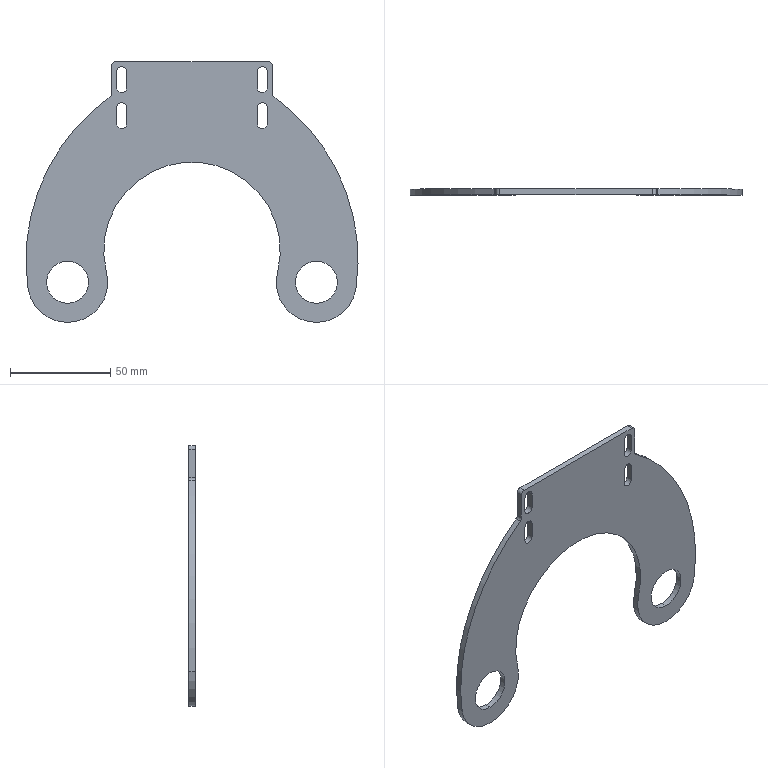Part | 1 solid | 40 faces | box 165.52 x 3 x 130 mm | volume 31712 mm3 | cylinder 27 | plane 13 | commonest cylinder face diameters 5 x12 4 x4 21 x4 40 x4 200 x2 88 x1
STEP:
#1=CARTESIAN_POINT('',(5.,0.,-2.5));
#2=VERTEX_POINT('',#1);
#3=CARTESIAN_POINT('',(7.5,0.,-5.));
#4=VERTEX_POINT('',#3);
#5=CARTESIAN_POINT('',(5.,0.,-5.));
#6=DIRECTION('',(0.,1.,0.));
#7=DIRECTION('',(0.,0.,1.));
#8=AXIS2_PLACEMENT_3D('',#5,#6,#7);
#9=CIRCLE('',#8,2.5);
#10=EDGE_CURVE('',#2,#4,#9,.T.);
#11=ORIENTED_EDGE('',*,*,#10,.F.);
#12=CARTESIAN_POINT('',(5.,3.,-2.5));
#13=VERTEX_POINT('',#12);
#14=CARTESIAN_POINT('',(5.,0.,-2.5));
#15=DIRECTION('',(0.,1.,0.));
#16=VECTOR('',#15,1000.);
#17=LINE('',#14,#16);
#18=EDGE_CURVE('',#2,#13,#17,.T.);
#19=ORIENTED_EDGE('',*,*,#18,.T.);
#20=CARTESIAN_POINT('',(7.5,3.,-5.));
#21=VERTEX_POINT('',#20);
#22=CARTESIAN_POINT('',(5.,3.,-5.));
#23=DIRECTION('',(0.,1.,0.));
#24=DIRECTION('',(0.,0.,1.));
#25=AXIS2_PLACEMENT_3D('',#22,#23,#24);
#26=CIRCLE('',#25,2.5);
#27=EDGE_CURVE('',#13,#21,#26,.T.);
#28=ORIENTED_EDGE('',*,*,#27,.T.);
#29=CARTESIAN_POINT('',(7.5,0.,-5.));
#30=DIRECTION('',(0.,1.,0.));
#31=VECTOR('',#30,1000.);
#32=LINE('',#29,#31);
#33=EDGE_CURVE('',#4,#21,#32,.T.);
#34=ORIENTED_EDGE('',*,*,#33,.F.);
#35=EDGE_LOOP('',(#11,#19,#28,#34));
#36=FACE_OUTER_BOUND('',#35,.T.);
#37=CARTESIAN_POINT('',(5.,0.,-5.));
#38=DIRECTION('',(0.,1.,0.));
#39=DIRECTION('',(0.,0.,1.));
#40=AXIS2_PLACEMENT_3D('',#37,#38,#39);
#41=CYLINDRICAL_SURFACE('',#40,2.5);
#42=ADVANCED_FACE('',(#36),#41,.F.);
#43=CARTESIAN_POINT('',(75.,0.,-20.5));
#44=VERTEX_POINT('',#43);
#45=CARTESIAN_POINT('',(77.5,0.,-23.));
#46=VERTEX_POINT('',#45);
#47=CARTESIAN_POINT('',(75.,0.,-23.));
#48=DIRECTION('',(0.,1.,0.));
#49=DIRECTION('',(0.,0.,-1.));
#50=AXIS2_PLACEMENT_3D('',#47,#48,#49);
#51=CIRCLE('',#50,2.5);
#52=EDGE_CURVE('',#44,#46,#51,.T.);
#53=ORIENTED_EDGE('',*,*,#52,.F.);
#54=CARTESIAN_POINT('',(75.,3.,-20.5));
#55=VERTEX_POINT('',#54);
#56=CARTESIAN_POINT('',(75.,0.,-20.5));
#57=DIRECTION('',(0.,1.,0.));
#58=VECTOR('',#57,1000.);
#59=LINE('',#56,#58);
#60=EDGE_CURVE('',#44,#55,#59,.T.);
#61=ORIENTED_EDGE('',*,*,#60,.T.);
#62=CARTESIAN_POINT('',(77.5,3.,-23.));
#63=VERTEX_POINT('',#62);
#64=CARTESIAN_POINT('',(75.,3.,-23.));
#65=DIRECTION('',(0.,1.,0.));
#66=DIRECTION('',(0.,0.,-1.));
#67=AXIS2_PLACEMENT_3D('',#64,#65,#66);
#68=CIRCLE('',#67,2.5);
#69=EDGE_CURVE('',#55,#63,#68,.T.);
#70=ORIENTED_EDGE('',*,*,#69,.T.);
#71=CARTESIAN_POINT('',(77.5,0.,-23.));
#72=DIRECTION('',(0.,1.,0.));
#73=VECTOR('',#72,1000.);
#74=LINE('',#71,#73);
#75=EDGE_CURVE('',#46,#63,#74,.T.);
#76=ORIENTED_EDGE('',*,*,#75,.F.);
#77=EDGE_LOOP('',(#53,#61,#70,#76));
#78=FACE_OUTER_BOUND('',#77,.T.);
#79=CARTESIAN_POINT('',(75.,0.,-23.));
#80=DIRECTION('',(0.,1.,0.));
#81=DIRECTION('',(0.,0.,1.));
#82=AXIS2_PLACEMENT_3D('',#79,#80,#81);
#83=CYLINDRICAL_SURFACE('',#82,2.5);
#84=ADVANCED_FACE('',(#78),#83,.F.);
#85=CARTESIAN_POINT('',(75.,0.,-2.5));
#86=VERTEX_POINT('',#85);
#87=CARTESIAN_POINT('',(77.5,0.,-5.));
#88=VERTEX_POINT('',#87);
#89=CARTESIAN_POINT('',(75.,0.,-5.));
#90=DIRECTION('',(0.,1.,0.));
#91=DIRECTION('',(0.,0.,-1.));
#92=AXIS2_PLACEMENT_3D('',#89,#90,#91);
#93=CIRCLE('',#92,2.5);
#94=EDGE_CURVE('',#86,#88,#93,.T.);
#95=ORIENTED_EDGE('',*,*,#94,.F.);
#96=CARTESIAN_POINT('',(75.,3.,-2.5));
#97=VERTEX_POINT('',#96);
#98=CARTESIAN_POINT('',(75.,0.,-2.5));
#99=DIRECTION('',(0.,1.,0.));
#100=VECTOR('',#99,1000.);
#101=LINE('',#98,#100);
#102=EDGE_CURVE('',#86,#97,#101,.T.);
#103=ORIENTED_EDGE('',*,*,#102,.T.);
#104=CARTESIAN_POINT('',(77.5,3.,-5.));
#105=VERTEX_POINT('',#104);
#106=CARTESIAN_POINT('',(75.,3.,-5.));
#107=DIRECTION('',(0.,1.,0.));
#108=DIRECTION('',(0.,0.,-1.));
#109=AXIS2_PLACEMENT_3D('',#106,#107,#108);
#110=CIRCLE('',#109,2.5);
#111=EDGE_CURVE('',#97,#105,#110,.T.);
#112=ORIENTED_EDGE('',*,*,#111,.T.);
#113=CARTESIAN_POINT('',(77.5,0.,-5.));
#114=DIRECTION('',(0.,1.,0.));
#115=VECTOR('',#114,1000.);
#116=LINE('',#113,#115);
#117=EDGE_CURVE('',#88,#105,#116,.T.);
#118=ORIENTED_EDGE('',*,*,#117,.F.);
#119=EDGE_LOOP('',(#95,#103,#112,#118));
#120=FACE_OUTER_BOUND('',#119,.T.);
#121=CARTESIAN_POINT('',(75.,0.,-5.));
#122=DIRECTION('',(0.,1.,0.));
#123=DIRECTION('',(0.,0.,1.));
#124=AXIS2_PLACEMENT_3D('',#121,#122,#123);
#125=CYLINDRICAL_SURFACE('',#124,2.5);
#126=ADVANCED_FACE('',(#120),#125,.F.);
#127=CARTESIAN_POINT('',(5.,0.,-20.5));
#128=VERTEX_POINT('',#127);
#129=CARTESIAN_POINT('',(7.5,0.,-23.));
#130=VERTEX_POINT('',#129);
#131=CARTESIAN_POINT('',(5.,0.,-23.));
#132=DIRECTION('',(0.,1.,0.));
#133=DIRECTION('',(0.,0.,1.));
#134=AXIS2_PLACEMENT_3D('',#131,#132,#133);
#135=CIRCLE('',#134,2.5);
#136=EDGE_CURVE('',#128,#130,#135,.T.);
#137=ORIENTED_EDGE('',*,*,#136,.F.);
#138=CARTESIAN_POINT('',(5.,3.,-20.5));
#139=VERTEX_POINT('',#138);
#140=CARTESIAN_POINT('',(5.,0.,-20.5));
#141=DIRECTION('',(0.,1.,0.));
#142=VECTOR('',#141,1000.);
#143=LINE('',#140,#142);
#144=EDGE_CURVE('',#128,#139,#143,.T.);
#145=ORIENTED_EDGE('',*,*,#144,.T.);
#146=CARTESIAN_POINT('',(7.5,3.,-23.));
#147=VERTEX_POINT('',#146);
#148=CARTESIAN_POINT('',(5.,3.,-23.));
#149=DIRECTION('',(0.,1.,0.));
#150=DIRECTION('',(0.,0.,1.));
#151=AXIS2_PLACEMENT_3D('',#148,#149,#150);
#152=CIRCLE('',#151,2.5);
#153=EDGE_CURVE('',#139,#147,#152,.T.);
#154=ORIENTED_EDGE('',*,*,#153,.T.);
#155=CARTESIAN_POINT('',(7.5,0.,-23.));
#156=DIRECTION('',(0.,1.,0.));
#157=VECTOR('',#156,1000.);
#158=LINE('',#155,#157);
#159=EDGE_CURVE('',#130,#147,#158,.T.);
#160=ORIENTED_EDGE('',*,*,#159,.F.);
#161=EDGE_LOOP('',(#137,#145,#154,#160));
#162=FACE_OUTER_BOUND('',#161,.T.);
#163=CARTESIAN_POINT('',(5.,0.,-23.));
#164=DIRECTION('',(0.,1.,0.));
#165=DIRECTION('',(0.,0.,1.));
#166=AXIS2_PLACEMENT_3D('',#163,#164,#165);
#167=CYLINDRICAL_SURFACE('',#166,2.5);
#168=ADVANCED_FACE('',(#162),#167,.F.);
#169=CARTESIAN_POINT('',(-22.,0.,-120.5));
#170=VERTEX_POINT('',#169);
#171=CARTESIAN_POINT('',(-22.,0.,-99.5));
#172=VERTEX_POINT('',#171);
#173=CARTESIAN_POINT('',(-22.,0.,-110.));
#174=DIRECTION('',(0.,1.,0.));
#175=DIRECTION('',(0.,0.,1.));
#176=AXIS2_PLACEMENT_3D('',#173,#174,#175);
#177=CIRCLE('',#176,10.5);
#178=EDGE_CURVE('',#170,#172,#177,.T.);
#179=ORIENTED_EDGE('',*,*,#178,.F.);
#180=CARTESIAN_POINT('',(-22.,3.,-120.5));
#181=VERTEX_POINT('',#180);
#182=CARTESIAN_POINT('',(-22.,3.,-120.5));
#183=DIRECTION('',(0.,1.,0.));
#184=VECTOR('',#183,1000.);
#185=LINE('',#182,#184);
#186=EDGE_CURVE('',#170,#181,#185,.T.);
#187=ORIENTED_EDGE('',*,*,#186,.T.);
#188=CARTESIAN_POINT('',(-22.,3.,-99.5));
#189=VERTEX_POINT('',#188);
#190=CARTESIAN_POINT('',(-22.,3.,-110.));
#191=DIRECTION('',(0.,1.,0.));
#192=DIRECTION('',(0.,0.,1.));
#193=AXIS2_PLACEMENT_3D('',#190,#191,#192);
#194=CIRCLE('',#193,10.5);
#195=EDGE_CURVE('',#181,#189,#194,.T.);
#196=ORIENTED_EDGE('',*,*,#195,.T.);
#197=CARTESIAN_POINT('',(-22.,3.,-99.5));
#198=DIRECTION('',(0.,1.,0.));
#199=VECTOR('',#198,1000.);
#200=LINE('',#197,#199);
#201=EDGE_CURVE('',#172,#189,#200,.T.);
#202=ORIENTED_EDGE('',*,*,#201,.F.);
#203=EDGE_LOOP('',(#179,#187,#196,#202));
#204=FACE_OUTER_BOUND('',#203,.T.);
#205=CARTESIAN_POINT('',(-22.,3.,-110.));
#206=DIRECTION('',(0.,1.,0.));
#207=DIRECTION('',(0.,0.,1.));
#208=AXIS2_PLACEMENT_3D('',#205,#206,#207);
#209=CYLINDRICAL_SURFACE('',#208,10.5);
#210=ADVANCED_FACE('',(#204),#209,.F.);
#211=CARTESIAN_POINT('',(102.,0.,-120.5));
#212=VERTEX_POINT('',#211);
#213=CARTESIAN_POINT('',(102.,0.,-99.5));
#214=VERTEX_POINT('',#213);
#215=CARTESIAN_POINT('',(102.,0.,-110.));
#216=DIRECTION('',(0.,1.,0.));
#217=DIRECTION('',(0.,0.,1.));
#218=AXIS2_PLACEMENT_3D('',#215,#216,#217);
#219=CIRCLE('',#218,10.5);
#220=EDGE_CURVE('',#212,#214,#219,.T.);
#221=ORIENTED_EDGE('',*,*,#220,.F.);
#222=CARTESIAN_POINT('',(102.,3.,-120.5));
#223=VERTEX_POINT('',#222);
#224=CARTESIAN_POINT('',(102.,3.,-120.5));
#225=DIRECTION('',(0.,1.,0.));
#226=VECTOR('',#225,1000.);
#227=LINE('',#224,#226);
#228=EDGE_CURVE('',#212,#223,#227,.T.);
#229=ORIENTED_EDGE('',*,*,#228,.T.);
#230=CARTESIAN_POINT('',(102.,3.,-99.5));
#231=VERTEX_POINT('',#230);
#232=CARTESIAN_POINT('',(102.,3.,-110.));
#233=DIRECTION('',(0.,1.,0.));
#234=DIRECTION('',(0.,0.,1.));
#235=AXIS2_PLACEMENT_3D('',#232,#233,#234);
#236=CIRCLE('',#235,10.5);
#237=EDGE_CURVE('',#223,#231,#236,.T.);
#238=ORIENTED_EDGE('',*,*,#237,.T.);
#239=CARTESIAN_POINT('',(102.,3.,-99.5));
#240=DIRECTION('',(0.,1.,0.));
#241=VECTOR('',#240,1000.);
#242=LINE('',#239,#241);
#243=EDGE_CURVE('',#214,#231,#242,.T.);
#244=ORIENTED_EDGE('',*,*,#243,.F.);
#245=EDGE_LOOP('',(#221,#229,#238,#244));
#246=FACE_OUTER_BOUND('',#245,.T.);
#247=CARTESIAN_POINT('',(102.,3.,-110.));
#248=DIRECTION('',(0.,1.,0.));
#249=DIRECTION('',(0.,0.,1.));
#250=AXIS2_PLACEMENT_3D('',#247,#248,#249);
#251=CYLINDRICAL_SURFACE('',#250,10.5);
#252=ADVANCED_FACE('',(#246),#251,.F.);
#253=CARTESIAN_POINT('',(-22.,3.,-130.));
#254=VERTEX_POINT('',#253);
#255=CARTESIAN_POINT('',(-41.81,3.,-112.751));
#256=VERTEX_POINT('',#255);
#257=CARTESIAN_POINT('',(-22.,3.,-110.));
#258=DIRECTION('',(0.,1.,0.));
#259=DIRECTION('',(0.,0.,1.));
#260=AXIS2_PLACEMENT_3D('',#257,#258,#259);
#261=CIRCLE('',#260,20.);
#262=EDGE_CURVE('',#254,#256,#261,.T.);
#263=ORIENTED_EDGE('',*,*,#262,.F.);
#264=CARTESIAN_POINT('',(-22.,0.,-130.));
#265=VERTEX_POINT('',#264);
#266=CARTESIAN_POINT('',(-22.,3.,-130.));
#267=DIRECTION('',(0.,-1.,0.));
#268=VECTOR('',#267,1000.);
#269=LINE('',#266,#268);
#270=EDGE_CURVE('',#254,#265,#269,.T.);
#271=ORIENTED_EDGE('',*,*,#270,.T.);
#272=CARTESIAN_POINT('',(-41.81,0.,-112.751));
#273=VERTEX_POINT('',#272);
#274=CARTESIAN_POINT('',(-22.,0.,-110.));
#275=DIRECTION('',(0.,1.,0.));
#276=DIRECTION('',(0.,0.,1.));
#277=AXIS2_PLACEMENT_3D('',#274,#275,#276);
#278=CIRCLE('',#277,20.);
#279=EDGE_CURVE('',#265,#273,#278,.T.);
#280=ORIENTED_EDGE('',*,*,#279,.T.);
#281=CARTESIAN_POINT('',(-41.81,3.,-112.751));
#282=DIRECTION('',(0.,-1.,0.));
#283=VECTOR('',#282,1000.);
#284=LINE('',#281,#283);
#285=EDGE_CURVE('',#256,#273,#284,.T.);
#286=ORIENTED_EDGE('',*,*,#285,.F.);
#287=EDGE_LOOP('',(#263,#271,#280,#286));
#288=FACE_OUTER_BOUND('',#287,.T.);
#289=CARTESIAN_POINT('',(-22.,3.,-110.));
#290=DIRECTION('',(0.,-1.,0.));
#291=DIRECTION('',(0.,0.,-1.));
#292=AXIS2_PLACEMENT_3D('',#289,#290,#291);
#293=CYLINDRICAL_SURFACE('',#292,20.);
#294=ADVANCED_FACE('',(#288),#293,.T.);
#295=CARTESIAN_POINT('',(102.,3.,-130.));
#296=VERTEX_POINT('',#295);
#297=CARTESIAN_POINT('',(82.625,3.,-105.039));
#298=VERTEX_POINT('',#297);
#299=CARTESIAN_POINT('',(102.,3.,-110.));
#300=DIRECTION('',(0.,1.,0.));
#301=DIRECTION('',(0.,0.,-1.));
#302=AXIS2_PLACEMENT_3D('',#299,#300,#301);
#303=CIRCLE('',#302,20.);
#304=EDGE_CURVE('',#296,#298,#303,.T.);
#305=ORIENTED_EDGE('',*,*,#304,.F.);
#306=CARTESIAN_POINT('',(102.,0.,-130.));
#307=VERTEX_POINT('',#306);
#308=CARTESIAN_POINT('',(102.,3.,-130.));
#309=DIRECTION('',(0.,-1.,0.));
#310=VECTOR('',#309,1000.);
#311=LINE('',#308,#310);
#312=EDGE_CURVE('',#296,#307,#311,.T.);
#313=ORIENTED_EDGE('',*,*,#312,.T.);
#314=CARTESIAN_POINT('',(82.625,0.,-105.039));
#315=VERTEX_POINT('',#314);
#316=CARTESIAN_POINT('',(102.,0.,-110.));
#317=DIRECTION('',(0.,1.,0.));
#318=DIRECTION('',(0.,0.,-1.));
#319=AXIS2_PLACEMENT_3D('',#316,#317,#318);
#320=CIRCLE('',#319,20.);
#321=EDGE_CURVE('',#307,#315,#320,.T.);
#322=ORIENTED_EDGE('',*,*,#321,.T.);
#323=CARTESIAN_POINT('',(82.625,3.,-105.039));
#324=DIRECTION('',(0.,-1.,0.));
#325=VECTOR('',#324,1000.);
#326=LINE('',#323,#325);
#327=EDGE_CURVE('',#298,#315,#326,.T.);
#328=ORIENTED_EDGE('',*,*,#327,.F.);
#329=EDGE_LOOP('',(#305,#313,#322,#328));
#330=FACE_OUTER_BOUND('',#329,.T.);
#331=CARTESIAN_POINT('',(102.,3.,-110.));
#332=DIRECTION('',(0.,-1.,0.));
#333=DIRECTION('',(0.,0.,-1.));
#334=AXIS2_PLACEMENT_3D('',#331,#332,#333);
#335=CYLINDRICAL_SURFACE('',#334,20.);
#336=ADVANCED_FACE('',(#330),#335,.T.);
#337=CARTESIAN_POINT('',(0.,0.,-15.964));
#338=VERTEX_POINT('',#337);
#339=CARTESIAN_POINT('',(0.,0.,-2.));
#340=VERTEX_POINT('',#339);
#341=CARTESIAN_POINT('',(0.,0.,0.));
#342=DIRECTION('',(0.,0.,1.));
#343=VECTOR('',#342,1000.);
#344=LINE('',#341,#343);
#345=EDGE_CURVE('',#338,#340,#344,.T.);
#346=ORIENTED_EDGE('',*,*,#345,.T.);
#347=CARTESIAN_POINT('',(0.,3.,-2.));
#348=VERTEX_POINT('',#347);
#349=CARTESIAN_POINT('',(0.,3.,-2.));
#350=DIRECTION('',(0.,1.,0.));
#351=VECTOR('',#350,1000.);
#352=LINE('',#349,#351);
#353=EDGE_CURVE('',#340,#348,#352,.T.);
#354=ORIENTED_EDGE('',*,*,#353,.T.);
#355=CARTESIAN_POINT('',(0.,3.,-15.964));
#356=VERTEX_POINT('',#355);
#357=CARTESIAN_POINT('',(0.,3.,0.));
#358=DIRECTION('',(0.,0.,1.));
#359=VECTOR('',#358,1000.);
#360=LINE('',#357,#359);
#361=EDGE_CURVE('',#356,#348,#360,.T.);
#362=ORIENTED_EDGE('',*,*,#361,.F.);
#363=CARTESIAN_POINT('',(0.,0.,-15.964));
#364=DIRECTION('',(0.,-1.,0.));
#365=VECTOR('',#364,1000.);
#366=LINE('',#363,#365);
#367=EDGE_CURVE('',#356,#338,#366,.T.);
#368=ORIENTED_EDGE('',*,*,#367,.T.);
#369=EDGE_LOOP('',(#346,#354,#362,#368));
#370=FACE_OUTER_BOUND('',#369,.T.);
#371=CARTESIAN_POINT('',(0.,3.,0.));
#372=DIRECTION('',(1.,0.,0.));
#373=DIRECTION('',(0.,0.,-1.));
#374=AXIS2_PLACEMENT_3D('',#371,#372,#373);
#375=PLANE('',#374);
#376=ADVANCED_FACE('',(#370),#375,.F.);
#377=CARTESIAN_POINT('',(2.,0.,0.));
#378=VERTEX_POINT('',#377);
#379=CARTESIAN_POINT('',(78.,0.,0.));
#380=VERTEX_POINT('',#379);
#381=CARTESIAN_POINT('',(0.,0.,0.));
#382=DIRECTION('',(1.,0.,0.));
#383=VECTOR('',#382,1000.);
#384=LINE('',#381,#383);
#385=EDGE_CURVE('',#378,#380,#384,.T.);
#386=ORIENTED_EDGE('',*,*,#385,.T.);
#387=CARTESIAN_POINT('',(78.,3.,0.));
#388=VERTEX_POINT('',#387);
#389=CARTESIAN_POINT('',(78.,3.,0.));
#390=DIRECTION('',(0.,1.,0.));
#391=VECTOR('',#390,1000.);
#392=LINE('',#389,#391);
#393=EDGE_CURVE('',#380,#388,#392,.T.);
#394=ORIENTED_EDGE('',*,*,#393,.T.);
#395=CARTESIAN_POINT('',(2.,3.,0.));
#396=VERTEX_POINT('',#395);
#397=CARTESIAN_POINT('',(0.,3.,0.));
#398=DIRECTION('',(1.,0.,0.));
#399=VECTOR('',#398,1000.);
#400=LINE('',#397,#399);
#401=EDGE_CURVE('',#396,#388,#400,.T.);
#402=ORIENTED_EDGE('',*,*,#401,.F.);
#403=CARTESIAN_POINT('',(2.,3.,0.));
#404=DIRECTION('',(0.,-1.,0.));
#405=VECTOR('',#404,1000.);
#406=LINE('',#403,#405);
#407=EDGE_CURVE('',#396,#378,#406,.T.);
#408=ORIENTED_EDGE('',*,*,#407,.T.);
#409=EDGE_LOOP('',(#386,#394,#402,#408));
#410=FACE_OUTER_BOUND('',#409,.T.);
#411=CARTESIAN_POINT('',(0.,3.,0.));
#412=DIRECTION('',(0.,0.,-1.));
#413=DIRECTION('',(-1.,0.,0.));
#414=AXIS2_PLACEMENT_3D('',#411,#412,#413);
#415=PLANE('',#414);
#416=ADVANCED_FACE('',(#410),#415,.F.);
#417=CARTESIAN_POINT('',(80.,0.,-2.));
#418=VERTEX_POINT('',#417);
#419=CARTESIAN_POINT('',(80.,0.,-15.964));
#420=VERTEX_POINT('',#419);
#421=CARTESIAN_POINT('',(80.,0.,0.));
#422=DIRECTION('',(0.,0.,-1.));
#423=VECTOR('',#422,1000.);
#424=LINE('',#421,#423);
#425=EDGE_CURVE('',#418,#420,#424,.T.);
#426=ORIENTED_EDGE('',*,*,#425,.T.);
#427=CARTESIAN_POINT('',(80.,3.,-15.964));
#428=VERTEX_POINT('',#427);
#429=CARTESIAN_POINT('',(80.,3.,-15.964));
#430=DIRECTION('',(0.,1.,0.));
#431=VECTOR('',#430,1000.);
#432=LINE('',#429,#431);
#433=EDGE_CURVE('',#420,#428,#432,.T.);
#434=ORIENTED_EDGE('',*,*,#433,.T.);
#435=CARTESIAN_POINT('',(80.,3.,-2.));
#436=VERTEX_POINT('',#435);
#437=CARTESIAN_POINT('',(80.,3.,0.));
#438=DIRECTION('',(0.,0.,-1.));
#439=VECTOR('',#438,1000.);
#440=LINE('',#437,#439);
#441=EDGE_CURVE('',#436,#428,#440,.T.);
#442=ORIENTED_EDGE('',*,*,#441,.F.);
#443=CARTESIAN_POINT('',(80.,3.,-2.));
#444=DIRECTION('',(0.,-1.,0.));
#445=VECTOR('',#444,1000.);
#446=LINE('',#443,#445);
#447=EDGE_CURVE('',#436,#418,#446,.T.);
#448=ORIENTED_EDGE('',*,*,#447,.T.);
#449=EDGE_LOOP('',(#426,#434,#442,#448));
#450=FACE_OUTER_BOUND('',#449,.T.);
#451=CARTESIAN_POINT('',(80.,3.,0.));
#452=DIRECTION('',(-1.,0.,0.));
#453=DIRECTION('',(0.,0.,1.));
#454=AXIS2_PLACEMENT_3D('',#451,#452,#453);
#455=PLANE('',#454);
#456=ADVANCED_FACE('',(#450),#455,.F.);
#457=CARTESIAN_POINT('',(80.838,3.,-17.592));
#458=VERTEX_POINT('',#457);
#459=CARTESIAN_POINT('',(121.81,3.,-112.751));
#460=VERTEX_POINT('',#459);
#461=CARTESIAN_POINT('',(22.76,3.,-98.998));
#462=DIRECTION('',(0.,1.,0.));
#463=DIRECTION('',(0.,0.,-1.));
#464=AXIS2_PLACEMENT_3D('',#461,#462,#463);
#465=CIRCLE('',#464,100.);
#466=EDGE_CURVE('',#458,#460,#465,.T.);
#467=ORIENTED_EDGE('',*,*,#466,.F.);
#468=CARTESIAN_POINT('',(80.838,0.,-17.592));
#469=VERTEX_POINT('',#468);
#470=CARTESIAN_POINT('',(80.838,3.,-17.592));
#471=DIRECTION('',(0.,-1.,0.));
#472=VECTOR('',#471,1000.);
#473=LINE('',#470,#472);
#474=EDGE_CURVE('',#458,#469,#473,.T.);
#475=ORIENTED_EDGE('',*,*,#474,.T.);
#476=CARTESIAN_POINT('',(121.81,0.,-112.751));
#477=VERTEX_POINT('',#476);
#478=CARTESIAN_POINT('',(22.76,0.,-98.998));
#479=DIRECTION('',(0.,1.,0.));
#480=DIRECTION('',(0.,0.,-1.));
#481=AXIS2_PLACEMENT_3D('',#478,#479,#480);
#482=CIRCLE('',#481,100.);
#483=EDGE_CURVE('',#469,#477,#482,.T.);
#484=ORIENTED_EDGE('',*,*,#483,.T.);
#485=CARTESIAN_POINT('',(121.81,3.,-112.751));
#486=DIRECTION('',(0.,-1.,0.));
#487=VECTOR('',#486,1000.);
#488=LINE('',#485,#487);
#489=EDGE_CURVE('',#460,#477,#488,.T.);
#490=ORIENTED_EDGE('',*,*,#489,.F.);
#491=EDGE_LOOP('',(#467,#475,#484,#490));
#492=FACE_OUTER_BOUND('',#491,.T.);
#493=CARTESIAN_POINT('',(22.76,3.,-98.998));
#494=DIRECTION('',(0.,-1.,0.));
#495=DIRECTION('',(0.,0.,-1.));
#496=AXIS2_PLACEMENT_3D('',#493,#494,#495);
#497=CYLINDRICAL_SURFACE('',#496,100.);
#498=ADVANCED_FACE('',(#492),#497,.T.);
#499=ORIENTED_EDGE('',*,*,#312,.F.);
#500=CARTESIAN_POINT('',(102.,3.,-110.));
#501=DIRECTION('',(0.,1.,0.));
#502=DIRECTION('',(0.,0.,-1.));
#503=AXIS2_PLACEMENT_3D('',#500,#501,#502);
#504=CIRCLE('',#503,20.);
#505=EDGE_CURVE('',#460,#296,#504,.T.);
#506=ORIENTED_EDGE('',*,*,#505,.F.);
#507=ORIENTED_EDGE('',*,*,#489,.T.);
#508=CARTESIAN_POINT('',(102.,0.,-110.));
#509=DIRECTION('',(0.,1.,0.));
#510=DIRECTION('',(0.,0.,-1.));
#511=AXIS2_PLACEMENT_3D('',#508,#509,#510);
#512=CIRCLE('',#511,20.);
#513=EDGE_CURVE('',#477,#307,#512,.T.);
#514=ORIENTED_EDGE('',*,*,#513,.T.);
#515=EDGE_LOOP('',(#499,#506,#507,#514));
#516=FACE_OUTER_BOUND('',#515,.T.);
#517=CARTESIAN_POINT('',(102.,3.,-110.));
#518=DIRECTION('',(0.,-1.,0.));
#519=DIRECTION('',(0.,0.,-1.));
#520=AXIS2_PLACEMENT_3D('',#517,#518,#519);
#521=CYLINDRICAL_SURFACE('',#520,20.);
#522=ADVANCED_FACE('',(#516),#521,.T.);
#523=CARTESIAN_POINT('',(-2.625,0.,-105.039));
#524=VERTEX_POINT('',#523);
#525=CARTESIAN_POINT('',(40.,0.,-94.125));
#526=DIRECTION('',(0.,-1.,0.));
#527=DIRECTION('',(0.,0.,1.));
#528=AXIS2_PLACEMENT_3D('',#525,#526,#527);
#529=CIRCLE('',#528,44.);
#530=EDGE_CURVE('',#315,#524,#529,.T.);
#531=ORIENTED_EDGE('',*,*,#530,.T.);
#532=CARTESIAN_POINT('',(-2.625,3.,-105.039));
#533=VERTEX_POINT('',#532);
#534=CARTESIAN_POINT('',(-2.625,3.,-105.039));
#535=DIRECTION('',(0.,-1.,0.));
#536=VECTOR('',#535,1000.);
#537=LINE('',#534,#536);
#538=EDGE_CURVE('',#533,#524,#537,.T.);
#539=ORIENTED_EDGE('',*,*,#538,.F.);
#540=CARTESIAN_POINT('',(40.,3.,-94.125));
#541=DIRECTION('',(0.,-1.,0.));
#542=DIRECTION('',(0.,0.,1.));
#543=AXIS2_PLACEMENT_3D('',#540,#541,#542);
#544=CIRCLE('',#543,44.);
#545=EDGE_CURVE('',#298,#533,#544,.T.);
#546=ORIENTED_EDGE('',*,*,#545,.F.);
#547=ORIENTED_EDGE('',*,*,#327,.T.);
#548=EDGE_LOOP('',(#531,#539,#546,#547));
#549=FACE_OUTER_BOUND('',#548,.T.);
#550=CARTESIAN_POINT('',(40.,3.,-94.125));
#551=DIRECTION('',(0.,-1.,0.));
#552=DIRECTION('',(0.,0.,-1.));
#553=AXIS2_PLACEMENT_3D('',#550,#551,#552);
#554=CYLINDRICAL_SURFACE('',#553,44.);
#555=ADVANCED_FACE('',(#549),#554,.F.);
#556=ORIENTED_EDGE('',*,*,#270,.F.);
#557=CARTESIAN_POINT('',(-22.,3.,-110.));
#558=DIRECTION('',(0.,1.,0.));
#559=DIRECTION('',(0.,0.,1.));
#560=AXIS2_PLACEMENT_3D('',#557,#558,#559);
#561=CIRCLE('',#560,20.);
#562=EDGE_CURVE('',#533,#254,#561,.T.);
#563=ORIENTED_EDGE('',*,*,#562,.F.);
#564=ORIENTED_EDGE('',*,*,#538,.T.);
#565=CARTESIAN_POINT('',(-22.,0.,-110.));
#566=DIRECTION('',(0.,1.,0.));
#567=DIRECTION('',(0.,0.,1.));
#568=AXIS2_PLACEMENT_3D('',#565,#566,#567);
#569=CIRCLE('',#568,20.);
#570=EDGE_CURVE('',#524,#265,#569,.T.);
#571=ORIENTED_EDGE('',*,*,#570,.T.);
#572=EDGE_LOOP('',(#556,#563,#564,#571));
#573=FACE_OUTER_BOUND('',#572,.T.);
#574=CARTESIAN_POINT('',(-22.,3.,-110.));
#575=DIRECTION('',(0.,-1.,0.));
#576=DIRECTION('',(0.,0.,-1.));
#577=AXIS2_PLACEMENT_3D('',#574,#575,#576);
#578=CYLINDRICAL_SURFACE('',#577,20.);
#579=ADVANCED_FACE('',(#573),#578,.T.);
#580=CARTESIAN_POINT('',(-0.8384,0.,-17.592));
#581=VERTEX_POINT('',#580);
#582=CARTESIAN_POINT('',(57.24,0.,-98.998));
#583=DIRECTION('',(0.,1.,0.));
#584=DIRECTION('',(0.,0.,1.));
#585=AXIS2_PLACEMENT_3D('',#582,#583,#584);
#586=CIRCLE('',#585,100.);
#587=EDGE_CURVE('',#273,#581,#586,.T.);
#588=ORIENTED_EDGE('',*,*,#587,.T.);
#589=CARTESIAN_POINT('',(-0.8384,3.,-17.592));
#590=VERTEX_POINT('',#589);
#591=CARTESIAN_POINT('',(-0.8384,3.,-17.592));
#592=DIRECTION('',(0.,1.,0.));
#593=VECTOR('',#592,1000.);
#594=LINE('',#591,#593);
#595=EDGE_CURVE('',#581,#590,#594,.T.);
#596=ORIENTED_EDGE('',*,*,#595,.T.);
#597=CARTESIAN_POINT('',(57.24,3.,-98.998));
#598=DIRECTION('',(0.,1.,0.));
#599=DIRECTION('',(0.,0.,1.));
#600=AXIS2_PLACEMENT_3D('',#597,#598,#599);
#601=CIRCLE('',#600,100.);
#602=EDGE_CURVE('',#256,#590,#601,.T.);
#603=ORIENTED_EDGE('',*,*,#602,.F.);
#604=ORIENTED_EDGE('',*,*,#285,.T.);
#605=EDGE_LOOP('',(#588,#596,#603,#604));
#606=FACE_OUTER_BOUND('',#605,.T.);
#607=CARTESIAN_POINT('',(57.24,3.,-98.998));
#608=DIRECTION('',(0.,-1.,0.));
#609=DIRECTION('',(0.,0.,-1.));
#610=AXIS2_PLACEMENT_3D('',#607,#608,#609);
#611=CYLINDRICAL_SURFACE('',#610,100.);
#612=ADVANCED_FACE('',(#606),#611,.T.);
#613=CARTESIAN_POINT('',(7.5,3.,-13.));
#614=VERTEX_POINT('',#613);
#615=CARTESIAN_POINT('',(2.5,3.,-13.));
#616=VERTEX_POINT('',#615);
#617=CARTESIAN_POINT('',(5.,3.,-13.));
#618=DIRECTION('',(0.,1.,0.));
#619=DIRECTION('',(0.,0.,1.));
#620=AXIS2_PLACEMENT_3D('',#617,#618,#619);
#621=CIRCLE('',#620,2.5);
#622=EDGE_CURVE('',#614,#616,#621,.T.);
#623=ORIENTED_EDGE('',*,*,#622,.F.);
#624=CARTESIAN_POINT('',(7.5,3.,-13.));
#625=DIRECTION('',(0.,0.,-1.));
#626=VECTOR('',#625,1000.);
#627=LINE('',#624,#626);
#628=EDGE_CURVE('',#21,#614,#627,.T.);
#629=ORIENTED_EDGE('',*,*,#628,.F.);
#630=ORIENTED_EDGE('',*,*,#27,.F.);
#631=CARTESIAN_POINT('',(2.5,3.,-5.));
#632=VERTEX_POINT('',#631);
#633=CARTESIAN_POINT('',(5.,3.,-5.));
#634=DIRECTION('',(0.,1.,0.));
#635=DIRECTION('',(0.,0.,1.));
#636=AXIS2_PLACEMENT_3D('',#633,#634,#635);
#637=CIRCLE('',#636,2.5);
#638=EDGE_CURVE('',#632,#13,#637,.T.);
#639=ORIENTED_EDGE('',*,*,#638,.F.);
#640=CARTESIAN_POINT('',(2.5,3.,-13.));
#641=DIRECTION('',(0.,0.,1.));
#642=VECTOR('',#641,1000.);
#643=LINE('',#640,#642);
#644=EDGE_CURVE('',#616,#632,#643,.T.);
#645=ORIENTED_EDGE('',*,*,#644,.F.);
#646=EDGE_LOOP('',(#623,#629,#630,#639,#645));
#647=FACE_BOUND('',#646,.T.);
#648=CARTESIAN_POINT('',(77.5,3.,-31.));
#649=VERTEX_POINT('',#648);
#650=CARTESIAN_POINT('',(72.5,3.,-31.));
#651=VERTEX_POINT('',#650);
#652=CARTESIAN_POINT('',(75.,3.,-31.));
#653=DIRECTION('',(0.,1.,0.));
#654=DIRECTION('',(0.,0.,-1.));
#655=AXIS2_PLACEMENT_3D('',#652,#653,#654);
#656=CIRCLE('',#655,2.5);
#657=EDGE_CURVE('',#649,#651,#656,.T.);
#658=ORIENTED_EDGE('',*,*,#657,.F.);
#659=CARTESIAN_POINT('',(77.5,3.,-31.));
#660=DIRECTION('',(0.,0.,-1.));
#661=VECTOR('',#660,1000.);
#662=LINE('',#659,#661);
#663=EDGE_CURVE('',#63,#649,#662,.T.);
#664=ORIENTED_EDGE('',*,*,#663,.F.);
#665=ORIENTED_EDGE('',*,*,#69,.F.);
#666=CARTESIAN_POINT('',(72.5,3.,-23.));
#667=VERTEX_POINT('',#666);
#668=CARTESIAN_POINT('',(75.,3.,-23.));
#669=DIRECTION('',(0.,1.,0.));
#670=DIRECTION('',(0.,0.,-1.));
#671=AXIS2_PLACEMENT_3D('',#668,#669,#670);
#672=CIRCLE('',#671,2.5);
#673=EDGE_CURVE('',#667,#55,#672,.T.);
#674=ORIENTED_EDGE('',*,*,#673,.F.);
#675=CARTESIAN_POINT('',(72.5,3.,-31.));
#676=DIRECTION('',(0.,0.,1.));
#677=VECTOR('',#676,1000.);
#678=LINE('',#675,#677);
#679=EDGE_CURVE('',#651,#667,#678,.T.);
#680=ORIENTED_EDGE('',*,*,#679,.F.);
#681=EDGE_LOOP('',(#658,#664,#665,#674,#680));
#682=FACE_BOUND('',#681,.T.);
#683=CARTESIAN_POINT('',(77.5,3.,-13.));
#684=VERTEX_POINT('',#683);
#685=CARTESIAN_POINT('',(72.5,3.,-13.));
#686=VERTEX_POINT('',#685);
#687=CARTESIAN_POINT('',(75.,3.,-13.));
#688=DIRECTION('',(0.,1.,0.));
#689=DIRECTION('',(0.,0.,-1.));
#690=AXIS2_PLACEMENT_3D('',#687,#688,#689);
#691=CIRCLE('',#690,2.5);
#692=EDGE_CURVE('',#684,#686,#691,.T.);
#693=ORIENTED_EDGE('',*,*,#692,.F.);
#694=CARTESIAN_POINT('',(77.5,3.,-13.));
#695=DIRECTION('',(0.,0.,-1.));
#696=VECTOR('',#695,1000.);
#697=LINE('',#694,#696);
#698=EDGE_CURVE('',#105,#684,#697,.T.);
#699=ORIENTED_EDGE('',*,*,#698,.F.);
#700=ORIENTED_EDGE('',*,*,#111,.F.);
#701=CARTESIAN_POINT('',(72.5,3.,-5.));
#702=VERTEX_POINT('',#701);
#703=CARTESIAN_POINT('',(75.,3.,-5.));
#704=DIRECTION('',(0.,1.,0.));
#705=DIRECTION('',(0.,0.,-1.));
#706=AXIS2_PLACEMENT_3D('',#703,#704,#705);
#707=CIRCLE('',#706,2.5);
#708=EDGE_CURVE('',#702,#97,#707,.T.);
#709=ORIENTED_EDGE('',*,*,#708,.F.);
#710=CARTESIAN_POINT('',(72.5,3.,-13.));
#711=DIRECTION('',(0.,0.,1.));
#712=VECTOR('',#711,1000.);
#713=LINE('',#710,#712);
#714=EDGE_CURVE('',#686,#702,#713,.T.);
#715=ORIENTED_EDGE('',*,*,#714,.F.);
#716=EDGE_LOOP('',(#693,#699,#700,#709,#715));
#717=FACE_BOUND('',#716,.T.);
#718=CARTESIAN_POINT('',(7.5,3.,-31.));
#719=VERTEX_POINT('',#718);
#720=CARTESIAN_POINT('',(2.5,3.,-31.));
#721=VERTEX_POINT('',#720);
#722=CARTESIAN_POINT('',(5.,3.,-31.));
#723=DIRECTION('',(0.,1.,0.));
#724=DIRECTION('',(0.,0.,1.));
#725=AXIS2_PLACEMENT_3D('',#722,#723,#724);
#726=CIRCLE('',#725,2.5);
#727=EDGE_CURVE('',#719,#721,#726,.T.);
#728=ORIENTED_EDGE('',*,*,#727,.F.);
#729=CARTESIAN_POINT('',(7.5,3.,-31.));
#730=DIRECTION('',(0.,0.,-1.));
#731=VECTOR('',#730,1000.);
#732=LINE('',#729,#731);
#733=EDGE_CURVE('',#147,#719,#732,.T.);
#734=ORIENTED_EDGE('',*,*,#733,.F.);
#735=ORIENTED_EDGE('',*,*,#153,.F.);
#736=CARTESIAN_POINT('',(2.5,3.,-23.));
#737=VERTEX_POINT('',#736);
#738=CARTESIAN_POINT('',(5.,3.,-23.));
#739=DIRECTION('',(0.,1.,0.));
#740=DIRECTION('',(0.,0.,1.));
#741=AXIS2_PLACEMENT_3D('',#738,#739,#740);
#742=CIRCLE('',#741,2.5);
#743=EDGE_CURVE('',#737,#139,#742,.T.);
#744=ORIENTED_EDGE('',*,*,#743,.F.);
#745=CARTESIAN_POINT('',(2.5,3.,-31.));
#746=DIRECTION('',(0.,0.,1.));
#747=VECTOR('',#746,1000.);
#748=LINE('',#745,#747);
#749=EDGE_CURVE('',#721,#737,#748,.T.);
#750=ORIENTED_EDGE('',*,*,#749,.F.);
#751=EDGE_LOOP('',(#728,#734,#735,#744,#750));
#752=FACE_BOUND('',#751,.T.);
#753=CARTESIAN_POINT('',(-22.,3.,-110.));
#754=DIRECTION('',(0.,1.,0.));
#755=DIRECTION('',(0.,0.,1.));
#756=AXIS2_PLACEMENT_3D('',#753,#754,#755);
#757=CIRCLE('',#756,10.5);
#758=EDGE_CURVE('',#189,#181,#757,.T.);
#759=ORIENTED_EDGE('',*,*,#758,.F.);
#760=ORIENTED_EDGE('',*,*,#195,.F.);
#761=EDGE_LOOP('',(#759,#760));
#762=FACE_BOUND('',#761,.T.);
#763=CARTESIAN_POINT('',(102.,3.,-110.));
#764=DIRECTION('',(0.,1.,0.));
#765=DIRECTION('',(0.,0.,1.));
#766=AXIS2_PLACEMENT_3D('',#763,#764,#765);
#767=CIRCLE('',#766,10.5);
#768=EDGE_CURVE('',#231,#223,#767,.T.);
#769=ORIENTED_EDGE('',*,*,#768,.F.);
#770=ORIENTED_EDGE('',*,*,#237,.F.);
#771=EDGE_LOOP('',(#769,#770));
#772=FACE_BOUND('',#771,.T.);
#773=ORIENTED_EDGE('',*,*,#401,.T.);
#774=CARTESIAN_POINT('',(78.,3.,-2.));
#775=DIRECTION('',(0.,1.,0.));
#776=DIRECTION('',(0.,0.,1.));
#777=AXIS2_PLACEMENT_3D('',#774,#775,#776);
#778=CIRCLE('',#777,2.);
#779=EDGE_CURVE('',#388,#436,#778,.T.);
#780=ORIENTED_EDGE('',*,*,#779,.T.);
#781=ORIENTED_EDGE('',*,*,#441,.T.);
#782=CARTESIAN_POINT('',(82.,3.,-15.964));
#783=DIRECTION('',(0.,-1.,0.));
#784=DIRECTION('',(0.,0.,1.));
#785=AXIS2_PLACEMENT_3D('',#782,#783,#784);
#786=CIRCLE('',#785,2.);
#787=EDGE_CURVE('',#428,#458,#786,.T.);
#788=ORIENTED_EDGE('',*,*,#787,.T.);
#789=ORIENTED_EDGE('',*,*,#466,.T.);
#790=ORIENTED_EDGE('',*,*,#505,.T.);
#791=ORIENTED_EDGE('',*,*,#304,.T.);
#792=ORIENTED_EDGE('',*,*,#545,.T.);
#793=ORIENTED_EDGE('',*,*,#562,.T.);
#794=ORIENTED_EDGE('',*,*,#262,.T.);
#795=ORIENTED_EDGE('',*,*,#602,.T.);
#796=CARTESIAN_POINT('',(-2.,3.,-15.964));
#797=DIRECTION('',(0.,-1.,0.));
#798=DIRECTION('',(0.,0.,1.));
#799=AXIS2_PLACEMENT_3D('',#796,#797,#798);
#800=CIRCLE('',#799,2.);
#801=EDGE_CURVE('',#590,#356,#800,.T.);
#802=ORIENTED_EDGE('',*,*,#801,.T.);
#803=ORIENTED_EDGE('',*,*,#361,.T.);
#804=CARTESIAN_POINT('',(2.,3.,-2.));
#805=DIRECTION('',(0.,1.,0.));
#806=DIRECTION('',(0.,0.,1.));
#807=AXIS2_PLACEMENT_3D('',#804,#805,#806);
#808=CIRCLE('',#807,2.);
#809=EDGE_CURVE('',#348,#396,#808,.T.);
#810=ORIENTED_EDGE('',*,*,#809,.T.);
#811=EDGE_LOOP('',(#773,#780,#781,#788,#789,#790,#791,#792,#793,#794,#795,#802,#803,#810));
#812=FACE_OUTER_BOUND('',#811,.T.);
#813=CARTESIAN_POINT('',(57.24,3.,-98.998));
#814=DIRECTION('',(0.,1.,0.));
#815=DIRECTION('',(0.,0.,1.));
#816=AXIS2_PLACEMENT_3D('',#813,#814,#815);
#817=PLANE('',#816);
#818=ADVANCED_FACE('',(#647,#682,#717,#752,#762,#772,#812),#817,.T.);
#819=CARTESIAN_POINT('',(7.5,0.,-13.));
#820=VERTEX_POINT('',#819);
#821=CARTESIAN_POINT('',(7.5,0.,-13.));
#822=DIRECTION('',(0.,0.,-1.));
#823=VECTOR('',#822,1000.);
#824=LINE('',#821,#823);
#825=EDGE_CURVE('',#4,#820,#824,.T.);
#826=ORIENTED_EDGE('',*,*,#825,.T.);
#827=CARTESIAN_POINT('',(2.5,0.,-13.));
#828=VERTEX_POINT('',#827);
#829=CARTESIAN_POINT('',(5.,0.,-13.));
#830=DIRECTION('',(0.,1.,0.));
#831=DIRECTION('',(0.,0.,1.));
#832=AXIS2_PLACEMENT_3D('',#829,#830,#831);
#833=CIRCLE('',#832,2.5);
#834=EDGE_CURVE('',#820,#828,#833,.T.);
#835=ORIENTED_EDGE('',*,*,#834,.T.);
#836=CARTESIAN_POINT('',(2.5,0.,-5.));
#837=VERTEX_POINT('',#836);
#838=CARTESIAN_POINT('',(2.5,0.,-13.));
#839=DIRECTION('',(0.,0.,1.));
#840=VECTOR('',#839,1000.);
#841=LINE('',#838,#840);
#842=EDGE_CURVE('',#828,#837,#841,.T.);
#843=ORIENTED_EDGE('',*,*,#842,.T.);
#844=CARTESIAN_POINT('',(5.,0.,-5.));
#845=DIRECTION('',(0.,1.,0.));
#846=DIRECTION('',(0.,0.,1.));
#847=AXIS2_PLACEMENT_3D('',#844,#845,#846);
#848=CIRCLE('',#847,2.5);
#849=EDGE_CURVE('',#837,#2,#848,.T.);
#850=ORIENTED_EDGE('',*,*,#849,.T.);
#851=ORIENTED_EDGE('',*,*,#10,.T.);
#852=EDGE_LOOP('',(#826,#835,#843,#850,#851));
#853=FACE_BOUND('',#852,.T.);
#854=CARTESIAN_POINT('',(77.5,0.,-31.));
#855=VERTEX_POINT('',#854);
#856=CARTESIAN_POINT('',(77.5,0.,-31.));
#857=DIRECTION('',(0.,0.,-1.));
#858=VECTOR('',#857,1000.);
#859=LINE('',#856,#858);
#860=EDGE_CURVE('',#46,#855,#859,.T.);
#861=ORIENTED_EDGE('',*,*,#860,.T.);
#862=CARTESIAN_POINT('',(72.5,0.,-31.));
#863=VERTEX_POINT('',#862);
#864=CARTESIAN_POINT('',(75.,0.,-31.));
#865=DIRECTION('',(0.,1.,0.));
#866=DIRECTION('',(0.,0.,-1.));
#867=AXIS2_PLACEMENT_3D('',#864,#865,#866);
#868=CIRCLE('',#867,2.5);
#869=EDGE_CURVE('',#855,#863,#868,.T.);
#870=ORIENTED_EDGE('',*,*,#869,.T.);
#871=CARTESIAN_POINT('',(72.5,0.,-23.));
#872=VERTEX_POINT('',#871);
#873=CARTESIAN_POINT('',(72.5,0.,-31.));
#874=DIRECTION('',(0.,0.,1.));
#875=VECTOR('',#874,1000.);
#876=LINE('',#873,#875);
#877=EDGE_CURVE('',#863,#872,#876,.T.);
#878=ORIENTED_EDGE('',*,*,#877,.T.);
#879=CARTESIAN_POINT('',(75.,0.,-23.));
#880=DIRECTION('',(0.,1.,0.));
#881=DIRECTION('',(0.,0.,-1.));
#882=AXIS2_PLACEMENT_3D('',#879,#880,#881);
#883=CIRCLE('',#882,2.5);
#884=EDGE_CURVE('',#872,#44,#883,.T.);
#885=ORIENTED_EDGE('',*,*,#884,.T.);
#886=ORIENTED_EDGE('',*,*,#52,.T.);
#887=EDGE_LOOP('',(#861,#870,#878,#885,#886));
#888=FACE_BOUND('',#887,.T.);
#889=CARTESIAN_POINT('',(77.5,0.,-13.));
#890=VERTEX_POINT('',#889);
#891=CARTESIAN_POINT('',(77.5,0.,-13.));
#892=DIRECTION('',(0.,0.,-1.));
#893=VECTOR('',#892,1000.);
#894=LINE('',#891,#893);
#895=EDGE_CURVE('',#88,#890,#894,.T.);
#896=ORIENTED_EDGE('',*,*,#895,.T.);
#897=CARTESIAN_POINT('',(72.5,0.,-13.));
#898=VERTEX_POINT('',#897);
#899=CARTESIAN_POINT('',(75.,0.,-13.));
#900=DIRECTION('',(0.,1.,0.));
#901=DIRECTION('',(0.,0.,-1.));
#902=AXIS2_PLACEMENT_3D('',#899,#900,#901);
#903=CIRCLE('',#902,2.5);
#904=EDGE_CURVE('',#890,#898,#903,.T.);
#905=ORIENTED_EDGE('',*,*,#904,.T.);
#906=CARTESIAN_POINT('',(72.5,0.,-5.));
#907=VERTEX_POINT('',#906);
#908=CARTESIAN_POINT('',(72.5,0.,-13.));
#909=DIRECTION('',(0.,0.,1.));
#910=VECTOR('',#909,1000.);
#911=LINE('',#908,#910);
#912=EDGE_CURVE('',#898,#907,#911,.T.);
#913=ORIENTED_EDGE('',*,*,#912,.T.);
#914=CARTESIAN_POINT('',(75.,0.,-5.));
#915=DIRECTION('',(0.,1.,0.));
#916=DIRECTION('',(0.,0.,-1.));
#917=AXIS2_PLACEMENT_3D('',#914,#915,#916);
#918=CIRCLE('',#917,2.5);
#919=EDGE_CURVE('',#907,#86,#918,.T.);
#920=ORIENTED_EDGE('',*,*,#919,.T.);
#921=ORIENTED_EDGE('',*,*,#94,.T.);
#922=EDGE_LOOP('',(#896,#905,#913,#920,#921));
#923=FACE_BOUND('',#922,.T.);
#924=CARTESIAN_POINT('',(7.5,0.,-31.));
#925=VERTEX_POINT('',#924);
#926=CARTESIAN_POINT('',(7.5,0.,-31.));
#927=DIRECTION('',(0.,0.,-1.));
#928=VECTOR('',#927,1000.);
#929=LINE('',#926,#928);
#930=EDGE_CURVE('',#130,#925,#929,.T.);
#931=ORIENTED_EDGE('',*,*,#930,.T.);
#932=CARTESIAN_POINT('',(2.5,0.,-31.));
#933=VERTEX_POINT('',#932);
#934=CARTESIAN_POINT('',(5.,0.,-31.));
#935=DIRECTION('',(0.,1.,0.));
#936=DIRECTION('',(0.,0.,1.));
#937=AXIS2_PLACEMENT_3D('',#934,#935,#936);
#938=CIRCLE('',#937,2.5);
#939=EDGE_CURVE('',#925,#933,#938,.T.);
#940=ORIENTED_EDGE('',*,*,#939,.T.);
#941=CARTESIAN_POINT('',(2.5,0.,-23.));
#942=VERTEX_POINT('',#941);
#943=CARTESIAN_POINT('',(2.5,0.,-31.));
#944=DIRECTION('',(0.,0.,1.));
#945=VECTOR('',#944,1000.);
#946=LINE('',#943,#945);
#947=EDGE_CURVE('',#933,#942,#946,.T.);
#948=ORIENTED_EDGE('',*,*,#947,.T.);
#949=CARTESIAN_POINT('',(5.,0.,-23.));
#950=DIRECTION('',(0.,1.,0.));
#951=DIRECTION('',(0.,0.,1.));
#952=AXIS2_PLACEMENT_3D('',#949,#950,#951);
#953=CIRCLE('',#952,2.5);
#954=EDGE_CURVE('',#942,#128,#953,.T.);
#955=ORIENTED_EDGE('',*,*,#954,.T.);
#956=ORIENTED_EDGE('',*,*,#136,.T.);
#957=EDGE_LOOP('',(#931,#940,#948,#955,#956));
#958=FACE_BOUND('',#957,.T.);
#959=CARTESIAN_POINT('',(-22.,0.,-110.));
#960=DIRECTION('',(0.,1.,0.));
#961=DIRECTION('',(0.,0.,1.));
#962=AXIS2_PLACEMENT_3D('',#959,#960,#961);
#963=CIRCLE('',#962,10.5);
#964=EDGE_CURVE('',#172,#170,#963,.T.);
#965=ORIENTED_EDGE('',*,*,#964,.T.);
#966=ORIENTED_EDGE('',*,*,#178,.T.);
#967=EDGE_LOOP('',(#965,#966));
#968=FACE_BOUND('',#967,.T.);
#969=CARTESIAN_POINT('',(102.,0.,-110.));
#970=DIRECTION('',(0.,1.,0.));
#971=DIRECTION('',(0.,0.,1.));
#972=AXIS2_PLACEMENT_3D('',#969,#970,#971);
#973=CIRCLE('',#972,10.5);
#974=EDGE_CURVE('',#214,#212,#973,.T.);
#975=ORIENTED_EDGE('',*,*,#974,.T.);
#976=ORIENTED_EDGE('',*,*,#220,.T.);
#977=EDGE_LOOP('',(#975,#976));
#978=FACE_BOUND('',#977,.T.);
#979=ORIENTED_EDGE('',*,*,#425,.F.);
#980=CARTESIAN_POINT('',(78.,0.,-2.));
#981=DIRECTION('',(0.,-1.,0.));
#982=DIRECTION('',(0.,0.,1.));
#983=AXIS2_PLACEMENT_3D('',#980,#981,#982);
#984=CIRCLE('',#983,2.);
#985=EDGE_CURVE('',#418,#380,#984,.T.);
#986=ORIENTED_EDGE('',*,*,#985,.T.);
#987=ORIENTED_EDGE('',*,*,#385,.F.);
#988=CARTESIAN_POINT('',(2.,0.,-2.));
#989=DIRECTION('',(0.,-1.,0.));
#990=DIRECTION('',(0.,0.,1.));
#991=AXIS2_PLACEMENT_3D('',#988,#989,#990);
#992=CIRCLE('',#991,2.);
#993=EDGE_CURVE('',#378,#340,#992,.T.);
#994=ORIENTED_EDGE('',*,*,#993,.T.);
#995=ORIENTED_EDGE('',*,*,#345,.F.);
#996=CARTESIAN_POINT('',(-2.,0.,-15.964));
#997=DIRECTION('',(0.,1.,0.));
#998=DIRECTION('',(0.,0.,1.));
#999=AXIS2_PLACEMENT_3D('',#996,#997,#998);
#1000=CIRCLE('',#999,2.);
#1001=EDGE_CURVE('',#338,#581,#1000,.T.);
#1002=ORIENTED_EDGE('',*,*,#1001,.T.);
#1003=ORIENTED_EDGE('',*,*,#587,.F.);
#1004=ORIENTED_EDGE('',*,*,#279,.F.);
#1005=ORIENTED_EDGE('',*,*,#570,.F.);
#1006=ORIENTED_EDGE('',*,*,#530,.F.);
#1007=ORIENTED_EDGE('',*,*,#321,.F.);
#1008=ORIENTED_EDGE('',*,*,#513,.F.);
#1009=ORIENTED_EDGE('',*,*,#483,.F.);
#1010=CARTESIAN_POINT('',(82.,0.,-15.964));
#1011=DIRECTION('',(0.,1.,0.));
#1012=DIRECTION('',(0.,0.,1.));
#1013=AXIS2_PLACEMENT_3D('',#1010,#1011,#1012);
#1014=CIRCLE('',#1013,2.);
#1015=EDGE_CURVE('',#469,#420,#1014,.T.);
#1016=ORIENTED_EDGE('',*,*,#1015,.T.);
#1017=EDGE_LOOP('',(#979,#986,#987,#994,#995,#1002,#1003,#1004,#1005,#1006,#1007,#1008,#1009,#1016));
#1018=FACE_OUTER_BOUND('',#1017,.T.);
#1019=CARTESIAN_POINT('',(57.24,0.,-98.998));
#1020=DIRECTION('',(0.,1.,0.));
#1021=DIRECTION('',(0.,0.,1.));
#1022=AXIS2_PLACEMENT_3D('',#1019,#1020,#1021);
#1023=PLANE('',#1022);
#1024=ADVANCED_FACE('',(#853,#888,#923,#958,#968,#978,#1018),#1023,.F.);
#1025=ORIENTED_EDGE('',*,*,#228,.F.);
#1026=ORIENTED_EDGE('',*,*,#974,.F.);
#1027=ORIENTED_EDGE('',*,*,#243,.T.);
#1028=ORIENTED_EDGE('',*,*,#768,.T.);
#1029=EDGE_LOOP('',(#1025,#1026,#1027,#1028));
#1030=FACE_OUTER_BOUND('',#1029,.T.);
#1031=CARTESIAN_POINT('',(102.,3.,-110.));
#1032=DIRECTION('',(0.,1.,0.));
#1033=DIRECTION('',(0.,0.,1.));
#1034=AXIS2_PLACEMENT_3D('',#1031,#1032,#1033);
#1035=CYLINDRICAL_SURFACE('',#1034,10.5);
#1036=ADVANCED_FACE('',(#1030),#1035,.F.);
#1037=ORIENTED_EDGE('',*,*,#186,.F.);
#1038=ORIENTED_EDGE('',*,*,#964,.F.);
#1039=ORIENTED_EDGE('',*,*,#201,.T.);
#1040=ORIENTED_EDGE('',*,*,#758,.T.);
#1041=EDGE_LOOP('',(#1037,#1038,#1039,#1040));
#1042=FACE_OUTER_BOUND('',#1041,.T.);
#1043=CARTESIAN_POINT('',(-22.,3.,-110.));
#1044=DIRECTION('',(0.,1.,0.));
#1045=DIRECTION('',(0.,0.,1.));
#1046=AXIS2_PLACEMENT_3D('',#1043,#1044,#1045);
#1047=CYLINDRICAL_SURFACE('',#1046,10.5);
#1048=ADVANCED_FACE('',(#1042),#1047,.F.);
#1049=ORIENTED_EDGE('',*,*,#727,.T.);
#1050=CARTESIAN_POINT('',(2.5,0.,-31.));
#1051=DIRECTION('',(0.,1.,0.));
#1052=VECTOR('',#1051,1000.);
#1053=LINE('',#1050,#1052);
#1054=EDGE_CURVE('',#933,#721,#1053,.T.);
#1055=ORIENTED_EDGE('',*,*,#1054,.F.);
#1056=ORIENTED_EDGE('',*,*,#939,.F.);
#1057=CARTESIAN_POINT('',(7.5,0.,-31.));
#1058=DIRECTION('',(0.,1.,0.));
#1059=VECTOR('',#1058,1000.);
#1060=LINE('',#1057,#1059);
#1061=EDGE_CURVE('',#925,#719,#1060,.T.);
#1062=ORIENTED_EDGE('',*,*,#1061,.T.);
#1063=EDGE_LOOP('',(#1049,#1055,#1056,#1062));
#1064=FACE_OUTER_BOUND('',#1063,.T.);
#1065=CARTESIAN_POINT('',(5.,0.,-31.));
#1066=DIRECTION('',(0.,1.,0.));
#1067=DIRECTION('',(0.,0.,1.));
#1068=AXIS2_PLACEMENT_3D('',#1065,#1066,#1067);
#1069=CYLINDRICAL_SURFACE('',#1068,2.5);
#1070=ADVANCED_FACE('',(#1064),#1069,.F.);
#1071=ORIENTED_EDGE('',*,*,#733,.T.);
#1072=ORIENTED_EDGE('',*,*,#1061,.F.);
#1073=ORIENTED_EDGE('',*,*,#930,.F.);
#1074=ORIENTED_EDGE('',*,*,#159,.T.);
#1075=EDGE_LOOP('',(#1071,#1072,#1073,#1074));
#1076=FACE_OUTER_BOUND('',#1075,.T.);
#1077=CARTESIAN_POINT('',(7.5,0.,-31.));
#1078=DIRECTION('',(1.,0.,0.));
#1079=DIRECTION('',(0.,0.,-1.));
#1080=AXIS2_PLACEMENT_3D('',#1077,#1078,#1079);
#1081=PLANE('',#1080);
#1082=ADVANCED_FACE('',(#1076),#1081,.F.);
#1083=ORIENTED_EDGE('',*,*,#144,.F.);
#1084=ORIENTED_EDGE('',*,*,#954,.F.);
#1085=CARTESIAN_POINT('',(2.5,0.,-23.));
#1086=DIRECTION('',(0.,1.,0.));
#1087=VECTOR('',#1086,1000.);
#1088=LINE('',#1085,#1087);
#1089=EDGE_CURVE('',#942,#737,#1088,.T.);
#1090=ORIENTED_EDGE('',*,*,#1089,.T.);
#1091=ORIENTED_EDGE('',*,*,#743,.T.);
#1092=EDGE_LOOP('',(#1083,#1084,#1090,#1091));
#1093=FACE_OUTER_BOUND('',#1092,.T.);
#1094=CARTESIAN_POINT('',(5.,0.,-23.));
#1095=DIRECTION('',(0.,1.,0.));
#1096=DIRECTION('',(0.,0.,1.));
#1097=AXIS2_PLACEMENT_3D('',#1094,#1095,#1096);
#1098=CYLINDRICAL_SURFACE('',#1097,2.5);
#1099=ADVANCED_FACE('',(#1093),#1098,.F.);
#1100=ORIENTED_EDGE('',*,*,#749,.T.);
#1101=ORIENTED_EDGE('',*,*,#1089,.F.);
#1102=ORIENTED_EDGE('',*,*,#947,.F.);
#1103=ORIENTED_EDGE('',*,*,#1054,.T.);
#1104=EDGE_LOOP('',(#1100,#1101,#1102,#1103));
#1105=FACE_OUTER_BOUND('',#1104,.T.);
#1106=CARTESIAN_POINT('',(2.5,0.,-31.));
#1107=DIRECTION('',(-1.,0.,0.));
#1108=DIRECTION('',(0.,0.,1.));
#1109=AXIS2_PLACEMENT_3D('',#1106,#1107,#1108);
#1110=PLANE('',#1109);
#1111=ADVANCED_FACE('',(#1105),#1110,.F.);
#1112=ORIENTED_EDGE('',*,*,#692,.T.);
#1113=CARTESIAN_POINT('',(72.5,0.,-13.));
#1114=DIRECTION('',(0.,1.,0.));
#1115=VECTOR('',#1114,1000.);
#1116=LINE('',#1113,#1115);
#1117=EDGE_CURVE('',#898,#686,#1116,.T.);
#1118=ORIENTED_EDGE('',*,*,#1117,.F.);
#1119=ORIENTED_EDGE('',*,*,#904,.F.);
#1120=CARTESIAN_POINT('',(77.5,0.,-13.));
#1121=DIRECTION('',(0.,1.,0.));
#1122=VECTOR('',#1121,1000.);
#1123=LINE('',#1120,#1122);
#1124=EDGE_CURVE('',#890,#684,#1123,.T.);
#1125=ORIENTED_EDGE('',*,*,#1124,.T.);
#1126=EDGE_LOOP('',(#1112,#1118,#1119,#1125));
#1127=FACE_OUTER_BOUND('',#1126,.T.);
#1128=CARTESIAN_POINT('',(75.,0.,-13.));
#1129=DIRECTION('',(0.,1.,0.));
#1130=DIRECTION('',(0.,0.,1.));
#1131=AXIS2_PLACEMENT_3D('',#1128,#1129,#1130);
#1132=CYLINDRICAL_SURFACE('',#1131,2.5);
#1133=ADVANCED_FACE('',(#1127),#1132,.F.);
#1134=ORIENTED_EDGE('',*,*,#698,.T.);
#1135=ORIENTED_EDGE('',*,*,#1124,.F.);
#1136=ORIENTED_EDGE('',*,*,#895,.F.);
#1137=ORIENTED_EDGE('',*,*,#117,.T.);
#1138=EDGE_LOOP('',(#1134,#1135,#1136,#1137));
#1139=FACE_OUTER_BOUND('',#1138,.T.);
#1140=CARTESIAN_POINT('',(77.5,0.,-13.));
#1141=DIRECTION('',(1.,0.,0.));
#1142=DIRECTION('',(0.,0.,-1.));
#1143=AXIS2_PLACEMENT_3D('',#1140,#1141,#1142);
#1144=PLANE('',#1143);
#1145=ADVANCED_FACE('',(#1139),#1144,.F.);
#1146=ORIENTED_EDGE('',*,*,#102,.F.);
#1147=ORIENTED_EDGE('',*,*,#919,.F.);
#1148=CARTESIAN_POINT('',(72.5,0.,-5.));
#1149=DIRECTION('',(0.,1.,0.));
#1150=VECTOR('',#1149,1000.);
#1151=LINE('',#1148,#1150);
#1152=EDGE_CURVE('',#907,#702,#1151,.T.);
#1153=ORIENTED_EDGE('',*,*,#1152,.T.);
#1154=ORIENTED_EDGE('',*,*,#708,.T.);
#1155=EDGE_LOOP('',(#1146,#1147,#1153,#1154));
#1156=FACE_OUTER_BOUND('',#1155,.T.);
#1157=CARTESIAN_POINT('',(75.,0.,-5.));
#1158=DIRECTION('',(0.,1.,0.));
#1159=DIRECTION('',(0.,0.,1.));
#1160=AXIS2_PLACEMENT_3D('',#1157,#1158,#1159);
#1161=CYLINDRICAL_SURFACE('',#1160,2.5);
#1162=ADVANCED_FACE('',(#1156),#1161,.F.);
#1163=ORIENTED_EDGE('',*,*,#714,.T.);
#1164=ORIENTED_EDGE('',*,*,#1152,.F.);
#1165=ORIENTED_EDGE('',*,*,#912,.F.);
#1166=ORIENTED_EDGE('',*,*,#1117,.T.);
#1167=EDGE_LOOP('',(#1163,#1164,#1165,#1166));
#1168=FACE_OUTER_BOUND('',#1167,.T.);
#1169=CARTESIAN_POINT('',(72.5,0.,-13.));
#1170=DIRECTION('',(-1.,0.,0.));
#1171=DIRECTION('',(0.,0.,1.));
#1172=AXIS2_PLACEMENT_3D('',#1169,#1170,#1171);
#1173=PLANE('',#1172);
#1174=ADVANCED_FACE('',(#1168),#1173,.F.);
#1175=ORIENTED_EDGE('',*,*,#657,.T.);
#1176=CARTESIAN_POINT('',(72.5,0.,-31.));
#1177=DIRECTION('',(0.,1.,0.));
#1178=VECTOR('',#1177,1000.);
#1179=LINE('',#1176,#1178);
#1180=EDGE_CURVE('',#863,#651,#1179,.T.);
#1181=ORIENTED_EDGE('',*,*,#1180,.F.);
#1182=ORIENTED_EDGE('',*,*,#869,.F.);
#1183=CARTESIAN_POINT('',(77.5,0.,-31.));
#1184=DIRECTION('',(0.,1.,0.));
#1185=VECTOR('',#1184,1000.);
#1186=LINE('',#1183,#1185);
#1187=EDGE_CURVE('',#855,#649,#1186,.T.);
#1188=ORIENTED_EDGE('',*,*,#1187,.T.);
#1189=EDGE_LOOP('',(#1175,#1181,#1182,#1188));
#1190=FACE_OUTER_BOUND('',#1189,.T.);
#1191=CARTESIAN_POINT('',(75.,0.,-31.));
#1192=DIRECTION('',(0.,1.,0.));
#1193=DIRECTION('',(0.,0.,1.));
#1194=AXIS2_PLACEMENT_3D('',#1191,#1192,#1193);
#1195=CYLINDRICAL_SURFACE('',#1194,2.5);
#1196=ADVANCED_FACE('',(#1190),#1195,.F.);
#1197=ORIENTED_EDGE('',*,*,#663,.T.);
#1198=ORIENTED_EDGE('',*,*,#1187,.F.);
#1199=ORIENTED_EDGE('',*,*,#860,.F.);
#1200=ORIENTED_EDGE('',*,*,#75,.T.);
#1201=EDGE_LOOP('',(#1197,#1198,#1199,#1200));
#1202=FACE_OUTER_BOUND('',#1201,.T.);
#1203=CARTESIAN_POINT('',(77.5,0.,-31.));
#1204=DIRECTION('',(1.,0.,0.));
#1205=DIRECTION('',(0.,0.,-1.));
#1206=AXIS2_PLACEMENT_3D('',#1203,#1204,#1205);
#1207=PLANE('',#1206);
#1208=ADVANCED_FACE('',(#1202),#1207,.F.);
#1209=ORIENTED_EDGE('',*,*,#60,.F.);
#1210=ORIENTED_EDGE('',*,*,#884,.F.);
#1211=CARTESIAN_POINT('',(72.5,0.,-23.));
#1212=DIRECTION('',(0.,1.,0.));
#1213=VECTOR('',#1212,1000.);
#1214=LINE('',#1211,#1213);
#1215=EDGE_CURVE('',#872,#667,#1214,.T.);
#1216=ORIENTED_EDGE('',*,*,#1215,.T.);
#1217=ORIENTED_EDGE('',*,*,#673,.T.);
#1218=EDGE_LOOP('',(#1209,#1210,#1216,#1217));
#1219=FACE_OUTER_BOUND('',#1218,.T.);
#1220=CARTESIAN_POINT('',(75.,0.,-23.));
#1221=DIRECTION('',(0.,1.,0.));
#1222=DIRECTION('',(0.,0.,1.));
#1223=AXIS2_PLACEMENT_3D('',#1220,#1221,#1222);
#1224=CYLINDRICAL_SURFACE('',#1223,2.5);
#1225=ADVANCED_FACE('',(#1219),#1224,.F.);
#1226=ORIENTED_EDGE('',*,*,#679,.T.);
#1227=ORIENTED_EDGE('',*,*,#1215,.F.);
#1228=ORIENTED_EDGE('',*,*,#877,.F.);
#1229=ORIENTED_EDGE('',*,*,#1180,.T.);
#1230=EDGE_LOOP('',(#1226,#1227,#1228,#1229));
#1231=FACE_OUTER_BOUND('',#1230,.T.);
#1232=CARTESIAN_POINT('',(72.5,0.,-31.));
#1233=DIRECTION('',(-1.,0.,0.));
#1234=DIRECTION('',(0.,0.,1.));
#1235=AXIS2_PLACEMENT_3D('',#1232,#1233,#1234);
#1236=PLANE('',#1235);
#1237=ADVANCED_FACE('',(#1231),#1236,.F.);
#1238=ORIENTED_EDGE('',*,*,#622,.T.);
#1239=CARTESIAN_POINT('',(2.5,0.,-13.));
#1240=DIRECTION('',(0.,1.,0.));
#1241=VECTOR('',#1240,1000.);
#1242=LINE('',#1239,#1241);
#1243=EDGE_CURVE('',#828,#616,#1242,.T.);
#1244=ORIENTED_EDGE('',*,*,#1243,.F.);
#1245=ORIENTED_EDGE('',*,*,#834,.F.);
#1246=CARTESIAN_POINT('',(7.5,0.,-13.));
#1247=DIRECTION('',(0.,1.,0.));
#1248=VECTOR('',#1247,1000.);
#1249=LINE('',#1246,#1248);
#1250=EDGE_CURVE('',#820,#614,#1249,.T.);
#1251=ORIENTED_EDGE('',*,*,#1250,.T.);
#1252=EDGE_LOOP('',(#1238,#1244,#1245,#1251));
#1253=FACE_OUTER_BOUND('',#1252,.T.);
#1254=CARTESIAN_POINT('',(5.,0.,-13.));
#1255=DIRECTION('',(0.,1.,0.));
#1256=DIRECTION('',(0.,0.,1.));
#1257=AXIS2_PLACEMENT_3D('',#1254,#1255,#1256);
#1258=CYLINDRICAL_SURFACE('',#1257,2.5);
#1259=ADVANCED_FACE('',(#1253),#1258,.F.);
#1260=ORIENTED_EDGE('',*,*,#628,.T.);
#1261=ORIENTED_EDGE('',*,*,#1250,.F.);
#1262=ORIENTED_EDGE('',*,*,#825,.F.);
#1263=ORIENTED_EDGE('',*,*,#33,.T.);
#1264=EDGE_LOOP('',(#1260,#1261,#1262,#1263));
#1265=FACE_OUTER_BOUND('',#1264,.T.);
#1266=CARTESIAN_POINT('',(7.5,0.,-13.));
#1267=DIRECTION('',(1.,0.,0.));
#1268=DIRECTION('',(0.,0.,-1.));
#1269=AXIS2_PLACEMENT_3D('',#1266,#1267,#1268);
#1270=PLANE('',#1269);
#1271=ADVANCED_FACE('',(#1265),#1270,.F.);
#1272=ORIENTED_EDGE('',*,*,#18,.F.);
#1273=ORIENTED_EDGE('',*,*,#849,.F.);
#1274=CARTESIAN_POINT('',(2.5,0.,-5.));
#1275=DIRECTION('',(0.,1.,0.));
#1276=VECTOR('',#1275,1000.);
#1277=LINE('',#1274,#1276);
#1278=EDGE_CURVE('',#837,#632,#1277,.T.);
#1279=ORIENTED_EDGE('',*,*,#1278,.T.);
#1280=ORIENTED_EDGE('',*,*,#638,.T.);
#1281=EDGE_LOOP('',(#1272,#1273,#1279,#1280));
#1282=FACE_OUTER_BOUND('',#1281,.T.);
#1283=CARTESIAN_POINT('',(5.,0.,-5.));
#1284=DIRECTION('',(0.,1.,0.));
#1285=DIRECTION('',(0.,0.,1.));
#1286=AXIS2_PLACEMENT_3D('',#1283,#1284,#1285);
#1287=CYLINDRICAL_SURFACE('',#1286,2.5);
#1288=ADVANCED_FACE('',(#1282),#1287,.F.);
#1289=ORIENTED_EDGE('',*,*,#644,.T.);
#1290=ORIENTED_EDGE('',*,*,#1278,.F.);
#1291=ORIENTED_EDGE('',*,*,#842,.F.);
#1292=ORIENTED_EDGE('',*,*,#1243,.T.);
#1293=EDGE_LOOP('',(#1289,#1290,#1291,#1292));
#1294=FACE_OUTER_BOUND('',#1293,.T.);
#1295=CARTESIAN_POINT('',(2.5,0.,-13.));
#1296=DIRECTION('',(-1.,0.,0.));
#1297=DIRECTION('',(0.,0.,1.));
#1298=AXIS2_PLACEMENT_3D('',#1295,#1296,#1297);
#1299=PLANE('',#1298);
#1300=ADVANCED_FACE('',(#1294),#1299,.F.);
#1301=ORIENTED_EDGE('',*,*,#787,.F.);
#1302=ORIENTED_EDGE('',*,*,#433,.F.);
#1303=ORIENTED_EDGE('',*,*,#1015,.F.);
#1304=ORIENTED_EDGE('',*,*,#474,.F.);
#1305=EDGE_LOOP('',(#1301,#1302,#1303,#1304));
#1306=FACE_OUTER_BOUND('',#1305,.T.);
#1307=CARTESIAN_POINT('',(82.,3.,-15.964));
#1308=DIRECTION('',(0.,-1.,0.));
#1309=DIRECTION('',(0.,0.,-1.));
#1310=AXIS2_PLACEMENT_3D('',#1307,#1308,#1309);
#1311=CYLINDRICAL_SURFACE('',#1310,2.);
#1312=ADVANCED_FACE('',(#1306),#1311,.F.);
#1313=ORIENTED_EDGE('',*,*,#779,.F.);
#1314=ORIENTED_EDGE('',*,*,#393,.F.);
#1315=ORIENTED_EDGE('',*,*,#985,.F.);
#1316=ORIENTED_EDGE('',*,*,#447,.F.);
#1317=EDGE_LOOP('',(#1313,#1314,#1315,#1316));
#1318=FACE_OUTER_BOUND('',#1317,.T.);
#1319=CARTESIAN_POINT('',(78.,3.,-2.));
#1320=DIRECTION('',(0.,-1.,0.));
#1321=DIRECTION('',(0.,0.,-1.));
#1322=AXIS2_PLACEMENT_3D('',#1319,#1320,#1321);
#1323=CYLINDRICAL_SURFACE('',#1322,2.);
#1324=ADVANCED_FACE('',(#1318),#1323,.T.);
#1325=ORIENTED_EDGE('',*,*,#809,.F.);
#1326=ORIENTED_EDGE('',*,*,#353,.F.);
#1327=ORIENTED_EDGE('',*,*,#993,.F.);
#1328=ORIENTED_EDGE('',*,*,#407,.F.);
#1329=EDGE_LOOP('',(#1325,#1326,#1327,#1328));
#1330=FACE_OUTER_BOUND('',#1329,.T.);
#1331=CARTESIAN_POINT('',(2.,3.,-2.));
#1332=DIRECTION('',(0.,-1.,0.));
#1333=DIRECTION('',(0.,0.,-1.));
#1334=AXIS2_PLACEMENT_3D('',#1331,#1332,#1333);
#1335=CYLINDRICAL_SURFACE('',#1334,2.);
#1336=ADVANCED_FACE('',(#1330),#1335,.T.);
#1337=ORIENTED_EDGE('',*,*,#801,.F.);
#1338=ORIENTED_EDGE('',*,*,#595,.F.);
#1339=ORIENTED_EDGE('',*,*,#1001,.F.);
#1340=ORIENTED_EDGE('',*,*,#367,.F.);
#1341=EDGE_LOOP('',(#1337,#1338,#1339,#1340));
#1342=FACE_OUTER_BOUND('',#1341,.T.);
#1343=CARTESIAN_POINT('',(-2.,3.,-15.964));
#1344=DIRECTION('',(0.,-1.,0.));
#1345=DIRECTION('',(0.,0.,-1.));
#1346=AXIS2_PLACEMENT_3D('',#1343,#1344,#1345);
#1347=CYLINDRICAL_SURFACE('',#1346,2.);
#1348=ADVANCED_FACE('',(#1342),#1347,.F.);
#1349=CLOSED_SHELL('',(#42,#84,#126,#168,#210,#252,#294,#336,#376,#416,#456,#498,#522,#555,#579,#612,#818,#1024,#1036,#1048,#1070,#1082,#1099,#1111,#1133,#1145,#1162,#1174,#1196,#1208,#1225,#1237,#1259,#1271,#1288,#1300,#1312,#1324,#1336,#1348));
#1350=MANIFOLD_SOLID_BREP('',#1349);
#1351=CARTESIAN_POINT('',(0.,0.,0.));
#1352=DIRECTION('',(0.,0.,1.));
#1353=DIRECTION('',(1.,0.,0.));
#1354=AXIS2_PLACEMENT_3D('',#1351,#1352,#1353);
#1355=(LENGTH_UNIT()NAMED_UNIT(*)SI_UNIT(.MILLI.,.METRE.));
#1356=UNCERTAINTY_MEASURE_WITH_UNIT(LENGTH_MEASURE(0.00001),#1355,'','');
#1357=(NAMED_UNIT(*)PLANE_ANGLE_UNIT()SI_UNIT($,.RADIAN.));
#1358=(NAMED_UNIT(*)SI_UNIT($,.STERADIAN.)SOLID_ANGLE_UNIT());
#1359=(GEOMETRIC_REPRESENTATION_CONTEXT(3)GLOBAL_UNCERTAINTY_ASSIGNED_CONTEXT((#1356))GLOBAL_UNIT_ASSIGNED_CONTEXT((#1355,#1357,#1358))REPRESENTATION_CONTEXT('',''));
#1360=ADVANCED_BREP_SHAPE_REPRESENTATION('',(#1350,#1354),#1359);